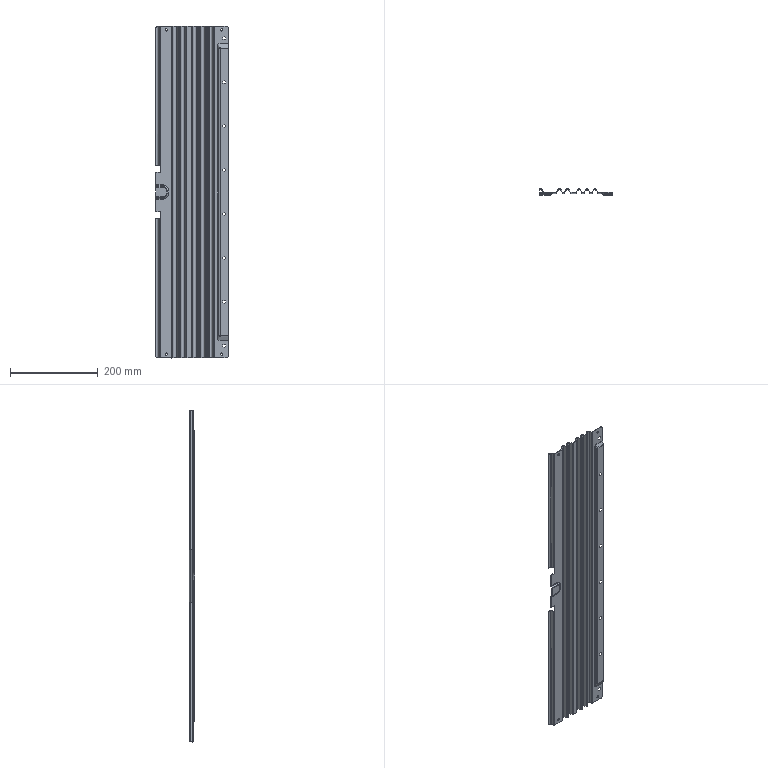Part | NX | features BREP 1 | 1 solid | 210 faces | box 165 x 13.655 x 755.2 mm | volume 191855 mm3 | plane 112 | cylinder 78 | torus 8 | cone 4 | spline 4 | sphere 4 | commonest cylinder face diameters 10 x11 1 x10 3.4 x10 5.1 x8 6 x8 7.6 x7